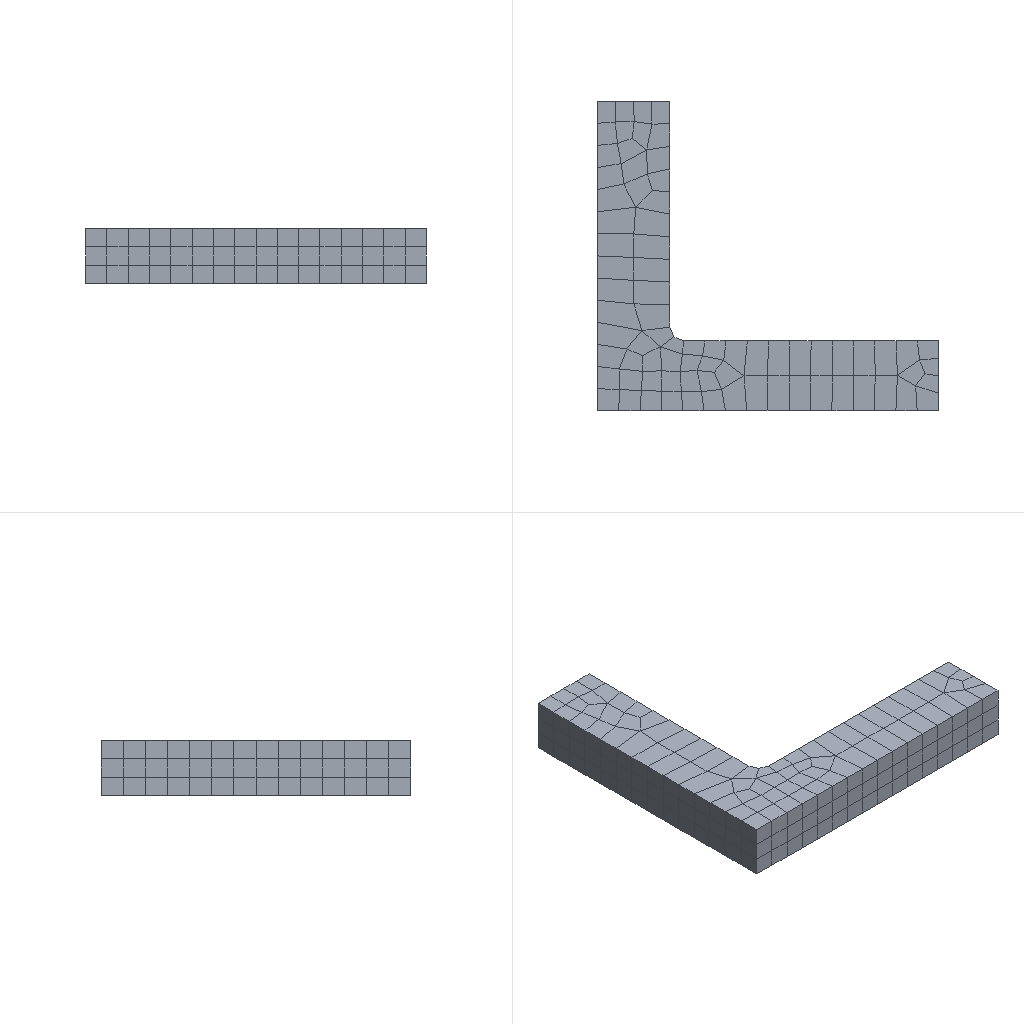Simulation study | ansys workbench
Set-up summary:
category,name,step,type,value,unit,region
solver,ansys_workbench
units,mm-N-s-tonne (MPa),,stated,"/units,MPA"
analysis,LS1,,static
load_step,LS1,LS1,static,nsubst=1; time=1
mesh,nodes,,,1473
mesh,elements,,,261
element_type,SOLID186,,,225
element_type,SURF154,,,36
material,Structural Steel,,E,200000,tonne s^-2 mm^-1
material,Structural Steel,,nu,0.3
material,Structural Steel,,density,7.85e-09,tonne mm^-3
material,Structural Steel,,conductivity,60.5,tonne mm s^-3 C^-1
material,Structural Steel,,specific_heat,4.34e+08,mm^2 s^-2 C^-1
material,Structural Steel,,cte,1.2e-05,C^-1
material,Structural Steel,,permeability,10000
material,Structural Steel,,resistivity,0.00017,ohm mm
load,Define Force Using Surface Effect Elements,LS1,surface-effect pres face 2,-3.611,,SURF154 #2
bc,Fixed Supports,model,fixed,[dofs=ALL],,_FIXEDSU
named_set,_FIXEDSU,,node,51
Ansys APDL input file, long lists of numbers shortened:
/batch
/config,noeldb,1     ! force off writing results to database
*get,_wallstrt,active,,time,wall
! ANSYS input file written by Workbench version 2022 R1
! File used for geometry attach:
/title,wbnew--____ (B5)
! ****** Begin Custom Load Command Snippet ******
/COM, ACT Extensions:
/COM,     LSDYNA, 2021.1
/COM,
! ****** End   Custom Load Command Snippet ******
*DIM,_wb_ProjectScratch_dir,string,248
_wb_ProjectScratch_dir(1) = ''
*DIM,_wb_SolverFiles_dir,string,248
_wb_SolverFiles_dir(1) = ''
*DIM,_wb_userfiles_dir,string,248
_wb_userfiles_dir(1) = ''
/com,--- Data in consistent NMM units. See Solving Units in the help system for more information.
/units,MPA
/nopr
/wb,file,start              !  signify a WB generated input file
/prep7
! Turn off shape checking because checks already performed inside WB mesher.
! See help system for more information.
SHPP,OFF,,NOWARN
/nolist
etcon,set             ! allow ANSYS to choose best KEYOP's for 180x elements, resets any applicable keyopt to MAPDL defaults
/com,*********** Nodes for the whole assembly ***********
nblock,3,,1620
(1i9,3e20.9e3)
        1     1.189067602E+01     7.367222271E+00     6.666666667E+00
! (1472 more lines like these left out)
-1
/wb,elem,start            !  set before creation of elements
/com,*********** Elements for Body 1 "__3333-FreeParts|NONE" ***********
et,1,186
keyo,1,2,1          ! set full integration on SOLID186
eblock,19,solid,,225
(19i9)
        1        1        1        1        0        0        0        0       20        0        1        3        5       77       13      134      133       97      129
! (449 more lines like these left out)
-1
/wb,elem,end               !  done creating elements
/com,*********** Send User Defined Coordinate System(s) ***********
csys,0
toffst,273.15,  ! Temperature offset from absolute zero
/com,*********** Set Reference Temperature ***********
tref,22.
/wb,mat,start              !  starting to send materials
/com,*********** Send Materials ***********
Temperature = 'TEMP' ! Temperature
MP,DENS,1,7.85e-09,	! tonne mm^-3
MP,ALPX,1,1.2e-05,	! C^-1
MP,C,1,434000000,	! mm^2 s^-2 C^-1
MP,KXX,1,60.5,	! tonne mm s^-3 C^-1
MP,RSVX,1,0.00017,	! ohm mm
MP,EX,1,200000,	! tonne s^-2 mm^-1
MP,NUXY,1,0.3,
MP,MURX,1,10000,
/wb,mat,end                !  done sending materials
!************************* Model Summary ********************
!__3333-FreeParts|NONE,	结构钢,	matid,	1
!************************* End Model Summary ********************
! get the diagonal of the bounding box. Needed later for other things
*get,_xmin,node,,mnloc,x
*get,_ymin,node,,mnloc,y
*get,_zmin,node,,mnloc,z
*get,_xmax,node,,mxloc,x
*get,_ymax,node,,mxloc,y
*get,_zmax,node,,mxloc,z
_ASMDIAG=(_xmax-_xmin)*(_xmax-_xmin)+(_ymax-_ymin)*(_ymax-_ymin)+(_zmax-_zmin)*(_zmax-_zmin)
_ASMDIAG=SQRT(_ASMDIAG)
/wb,contact,start          !  starting to send contact
/wb,contact,end            !  done creating contacts
/golist
/wb,load,start             !  starting to send loads
/com,*********** Fixed Supports ***********
CMBLOCK,_FIXEDSU,NODE,       51
(8i10)
       238       239       240       241       242       243       244       245
       246       247       248       249       250       251       252       253
       254       255       256       257      1155      1156      1157      1158
      1159      1160      1161      1162      1163      1164      1165      1166
      1167      1168      1169      1170      1171      1172      1173      1174
      1175      1176      1177      1178      1179      1180      1181      1182
      1184      1187      1189
cmsel,s,_FIXEDSU
d,all,all
nsel,all
/com,*********** Define Force Using Surface Effect Elements ***********
local,12,0,0.,0.,0.,0.,0.,0.
csys,0
et,2,154
eblock,10,,,36
(15i9)
      562        2        2        2       12      320      288      323      322     1244     1245     1302     1299
! (35 more lines like these left out)
-1
esel,s,type,,2
keyop,2,2,1                ! Apply load in local coordinate system
keyop,2,7,1                ! Use original area so load is constant in large deformation
esel,all
/gst,on,on
fini
*get,_numnode,node,0,count
*get,_numelem,elem,0,count
*get, _MAXELEMNUM, elem, 0, NUM, MAX
*get, _MAXNODENUM, node, 0, NUM, MAX
*get, _MAXELEMTYPE, etyp, 0, NUM, MAX
*get, _MAXREALCONST, real, 0, NUM, MAX
/go
/wb,load,end               !  done creating loads
/com,--- Number of total nodes = %_numnode%
/com,--- Number of contact elements = 36
/com,--- Number of spring elements = 0
/com,--- Number of bearing elements = 0
/com,--- Number of solid elements = 225
/com,--- Number of condensed parts = 0
/com,--- Number of total elements = %_numelem%
*get,_wallbsol,active,,time,wall
/com,****************************************************************************
/com,*************************    SOLUTION       ********************************
/com,****************************************************************************
/solu
antype,0                   ! static analysis
_thickRatio=  1     ! Ratio of thick parts in the model
eqsl,pcg,1e-8,,,,,,1
cntr,print,1               ! print out contact info and also make no initial contact an error
dmpoption,emat,no             ! Don't combine emat file for DANSYS
dmpoption,esav,no             ! Don't combine esav file for DANSYS
nldiag,cont,iter           ! print out contact info each equilibrium iteration
rescontrol,,none                 ! Do not keep any restart files
/com,****************************************************
/com,******************* SOLVE FOR LS 1 OF 1 ****************
esel,s,type,,2
nsle
sfe,all,1,pres,1,0.
sfe,all,2,pres,1,-3.611
sfe,all,3,pres,1,0.
nsel,all
esel,all
/nopr
/gopr
nsub,1,1,1
time,1.
outres,erase
outres,all,none
outres,nsol,all,
outres,rsol,all
outres,eangl,all
outres,etmp,all
outres,veng,all
outres,strs,all,
outres,epel,all,
outres,eppl,all,
outres,cont,all,
! *********** WB SOLVE COMMAND ***********
! check interactive state
*get,ANSINTER_,active,,int
*if,ANSINTER_,ne,0,then
/eof
*endif
solve
/com *************** Write FE CONNECTORS *********
CEWRITE,file,ce,,INTE
/com,****************************************************
/com,*************** FINISHED SOLVE FOR LS 1 *************
*get,_wallasol,active,,time,wall
/nopr
*get,_numnode,node,0,count
*get,_numelem,elem,0,count
*get, _MAXELEMNUM, elem, 0, NUM, MAX
*get, _MAXNODENUM, node, 0, NUM, MAX,,,INTERNAL
*get, _MAXELEMTYPE, etyp, 0, NUM, MAX
*get, _MAXREALCONST, real, 0, NUM, MAX
/gopr
*get,_PCGITER,active,,solu,cgiter
/post1
xmlo,ENCODING,ISO-8859-1
xmlo,parm
/xml,parm,xml
fini
/gopr
*get,_walldone,active,,time,wall
_preptime=(_wallbsol-_wallstrt)*3600
_solvtime=(_wallasol-_wallbsol)*3600
_posttime=(_walldone-_wallasol)*3600
_totaltim=(_walldone-_wallstrt)*3600
*get,_dlbratio,active,0,solu,dlbr
*get,_combtime,active,0,solu,comb
*get,_ssmode,active,0,solu,ssmm
*get,_ndofs,active,0,solu,ndof
*get,_sol_end_time,active,0,set,time
*if,_sol_end_time,eq,1.,then
/fclean				!clean distributed files
*endif
/com,--- Total number of nodes = %_numnode%
/com,--- Total number of elements = %_numelem%
/com,--- Element load balance ratio = %_dlbratio%
/com,--- Time to combine distributed files = %_combtime%
/com,--- Sparse memory mode = %_ssmode%
/com,--- Number of DOF = %_ndofs%
/wb,file,end               ! done with WB generated input
Results summary:
result,analyses[0].index,,,1
result,analyses[0].system,,,SYS
result,analyses[0].deck,,,deck.dat
result,analyses[0].solve_status,,,completed
result,analyses[0].analysis_type,,,static
result,analyses[0].physics,,,mechanical
result,analyses[0].unit_system,,,"NMM: mm, ton, N, s, mV, mA, degC"
result,analyses[0].n_sets,,,1
result,analyses[0].load_steps[0].set,set=1,,1
result,analyses[0].load_steps[0].time_or_freq,set=1,,1
result,analyses[0].load_steps[0].max_displacement_magnitude,set=1,,0.538
result,analyses[0].load_steps[0].max_von_mises_nodal,set=1,,310.291
result,analyses[0].load_steps[0].reaction_force_sum_xyz[1],set=1,,3.27897e-05
result,analyses[0].load_steps[0].reaction_force_sum_xyz[2],set=1,,1700
result,analyses[0].load_steps[0].reaction_force_sum_xyz[3],set=1,,-4.98588e-06